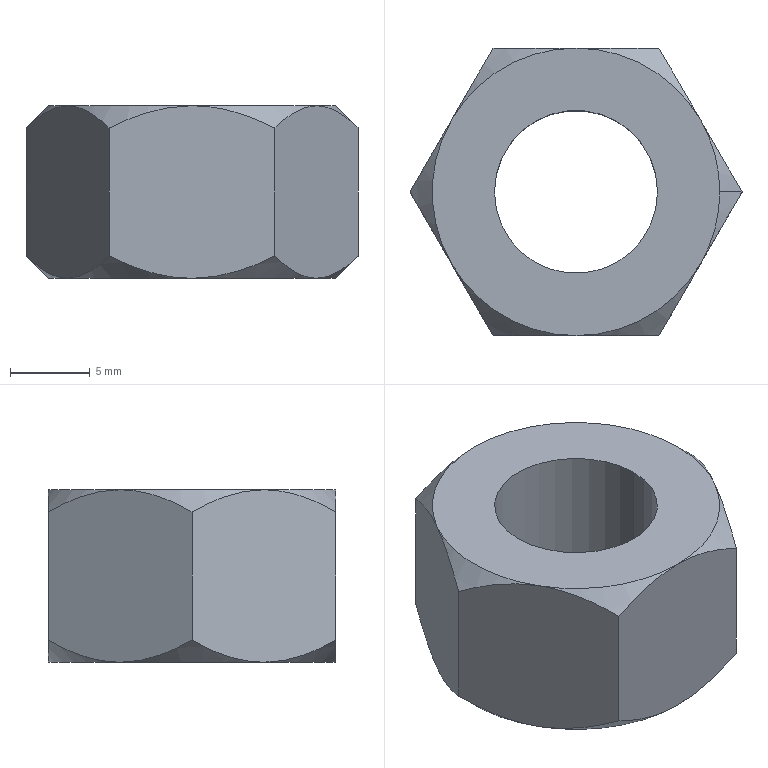Part | SolidWorks | features Extrusion 1, MirrorPattern 1, RevCutThin 1 | 1 solid | 24 faces | box 20.785 x 18 x 10.8 mm | volume 2126 mm3 | cone 14 | plane 8 | cylinder 2 | commonest cylinder face diameters 10.2 x2
STEP:
#1=CARTESIAN_POINT('',(9.,0.,10.8));
#2=VERTEX_POINT('',#1);
#3=CARTESIAN_POINT('',(7.794,4.5,10.8));
#4=VERTEX_POINT('',#3);
#5=CARTESIAN_POINT('',(0.,0.,10.8));
#6=DIRECTION('',(0.,0.,1.));
#7=DIRECTION('',(1.,0.,0.));
#8=AXIS2_PLACEMENT_3D('',#5,#6,#7);
#9=CIRCLE('',#8,9.);
#10=EDGE_CURVE('',#2,#4,#9,.T.);
#11=ORIENTED_EDGE('',*,*,#10,.F.);
#12=CARTESIAN_POINT('',(10.392,0.,9.408));
#13=VERTEX_POINT('',#12);
#14=CARTESIAN_POINT('',(9.,0.,10.8));
#15=DIRECTION('',(0.7071,0.,-0.7071));
#16=VECTOR('',#15,1000.);
#17=LINE('',#14,#16);
#18=EDGE_CURVE('',#2,#13,#17,.T.);
#19=ORIENTED_EDGE('',*,*,#18,.T.);
#20=CARTESIAN_POINT('',(7.794,4.5,10.8));
#21=CARTESIAN_POINT('',(8.246,3.717,10.8));
#22=CARTESIAN_POINT('',(8.69,2.948,10.662));
#23=CARTESIAN_POINT('',(9.566,1.43,10.164));
#24=CARTESIAN_POINT('',(9.985,0.7048,9.815));
#25=CARTESIAN_POINT('',(10.392,0.,9.408));
#26=B_SPLINE_CURVE_WITH_KNOTS('',3,(#20,#21,#22,#23,#24,#25),.UNSPECIFIED.,.F.,.F.,(4,2,4),(0.005387,0.008061,0.01074),.UNSPECIFIED.);
#27=EDGE_CURVE('',#4,#13,#26,.T.);
#28=ORIENTED_EDGE('',*,*,#27,.F.);
#29=EDGE_LOOP('',(#11,#19,#28));
#30=FACE_OUTER_BOUND('',#29,.T.);
#31=CARTESIAN_POINT('',(0.,0.,10.8));
#32=DIRECTION('',(0.,0.,-1.));
#33=DIRECTION('',(1.,0.,0.));
#34=AXIS2_PLACEMENT_3D('',#31,#32,#33);
#35=CONICAL_SURFACE('',#34,9.,0.7854);
#36=ADVANCED_FACE('',(#30),#35,.T.);
#37=CARTESIAN_POINT('',(7.794,-4.5,0.));
#38=VERTEX_POINT('',#37);
#39=CARTESIAN_POINT('',(9.,0.,0.));
#40=VERTEX_POINT('',#39);
#41=CARTESIAN_POINT('',(0.,0.,0.));
#42=DIRECTION('',(0.,0.,1.));
#43=DIRECTION('',(1.,0.,0.));
#44=AXIS2_PLACEMENT_3D('',#41,#42,#43);
#45=CIRCLE('',#44,9.);
#46=EDGE_CURVE('',#38,#40,#45,.T.);
#47=ORIENTED_EDGE('',*,*,#46,.T.);
#48=CARTESIAN_POINT('',(10.392,0.,1.392));
#49=VERTEX_POINT('',#48);
#50=CARTESIAN_POINT('',(9.,0.,0.));
#51=DIRECTION('',(0.7071,0.,0.7071));
#52=VECTOR('',#51,1000.);
#53=LINE('',#50,#52);
#54=EDGE_CURVE('',#40,#49,#53,.T.);
#55=ORIENTED_EDGE('',*,*,#54,.T.);
#56=CARTESIAN_POINT('',(7.794,-4.5,0.));
#57=CARTESIAN_POINT('',(8.246,-3.717,0.));
#58=CARTESIAN_POINT('',(8.69,-2.948,0.1382));
#59=CARTESIAN_POINT('',(9.566,-1.43,0.6363));
#60=CARTESIAN_POINT('',(9.985,-0.7048,0.9854));
#61=CARTESIAN_POINT('',(10.392,0.,1.392));
#62=B_SPLINE_CURVE_WITH_KNOTS('',3,(#56,#57,#58,#59,#60,#61),.UNSPECIFIED.,.F.,.F.,(4,2,4),(0.005387,0.008061,0.01074),.UNSPECIFIED.);
#63=EDGE_CURVE('',#38,#49,#62,.T.);
#64=ORIENTED_EDGE('',*,*,#63,.F.);
#65=EDGE_LOOP('',(#47,#55,#64));
#66=FACE_OUTER_BOUND('',#65,.T.);
#67=CARTESIAN_POINT('',(0.,0.,0.));
#68=DIRECTION('',(0.,0.,1.));
#69=DIRECTION('',(1.,0.,0.));
#70=AXIS2_PLACEMENT_3D('',#67,#68,#69);
#71=CONICAL_SURFACE('',#70,9.,0.7854);
#72=ADVANCED_FACE('',(#66),#71,.T.);
#73=CARTESIAN_POINT('',(-5.1,0.,10.8));
#74=VERTEX_POINT('',#73);
#75=CARTESIAN_POINT('',(5.1,0.,10.8));
#76=VERTEX_POINT('',#75);
#77=CARTESIAN_POINT('',(0.,0.,10.8));
#78=DIRECTION('',(0.,0.,1.));
#79=DIRECTION('',(1.,0.,0.));
#80=AXIS2_PLACEMENT_3D('',#77,#78,#79);
#81=CIRCLE('',#80,5.1);
#82=EDGE_CURVE('',#74,#76,#81,.T.);
#83=ORIENTED_EDGE('',*,*,#82,.T.);
#84=CARTESIAN_POINT('',(5.1,0.,0.));
#85=VERTEX_POINT('',#84);
#86=CARTESIAN_POINT('',(5.1,0.,10.8));
#87=DIRECTION('',(0.,0.,-1.));
#88=VECTOR('',#87,1000.);
#89=LINE('',#86,#88);
#90=EDGE_CURVE('',#76,#85,#89,.T.);
#91=ORIENTED_EDGE('',*,*,#90,.T.);
#92=CARTESIAN_POINT('',(-5.1,0.,0.));
#93=VERTEX_POINT('',#92);
#94=CARTESIAN_POINT('',(0.,0.,0.));
#95=DIRECTION('',(0.,0.,1.));
#96=DIRECTION('',(1.,0.,0.));
#97=AXIS2_PLACEMENT_3D('',#94,#95,#96);
#98=CIRCLE('',#97,5.1);
#99=EDGE_CURVE('',#93,#85,#98,.T.);
#100=ORIENTED_EDGE('',*,*,#99,.F.);
#101=CARTESIAN_POINT('',(-5.1,0.,10.8));
#102=DIRECTION('',(0.,0.,-1.));
#103=VECTOR('',#102,1000.);
#104=LINE('',#101,#103);
#105=EDGE_CURVE('',#74,#93,#104,.T.);
#106=ORIENTED_EDGE('',*,*,#105,.F.);
#107=EDGE_LOOP('',(#83,#91,#100,#106));
#108=FACE_OUTER_BOUND('',#107,.T.);
#109=CARTESIAN_POINT('',(0.,0.,10.8));
#110=DIRECTION('',(0.,0.,-1.));
#111=DIRECTION('',(-1.,0.,0.));
#112=AXIS2_PLACEMENT_3D('',#109,#110,#111);
#113=CYLINDRICAL_SURFACE('',#112,5.1);
#114=ADVANCED_FACE('',(#108),#113,.F.);
#115=CARTESIAN_POINT('',(0.,-9.,10.8));
#116=VERTEX_POINT('',#115);
#117=CARTESIAN_POINT('',(7.794,-4.5,10.8));
#118=VERTEX_POINT('',#117);
#119=CARTESIAN_POINT('',(0.,0.,10.8));
#120=DIRECTION('',(0.,0.,1.));
#121=DIRECTION('',(1.,0.,0.));
#122=AXIS2_PLACEMENT_3D('',#119,#120,#121);
#123=CIRCLE('',#122,9.);
#124=EDGE_CURVE('',#116,#118,#123,.T.);
#125=ORIENTED_EDGE('',*,*,#124,.T.);
#126=CARTESIAN_POINT('',(0.,0.,10.8));
#127=DIRECTION('',(0.,0.,1.));
#128=DIRECTION('',(1.,0.,0.));
#129=AXIS2_PLACEMENT_3D('',#126,#127,#128);
#130=CIRCLE('',#129,9.);
#131=EDGE_CURVE('',#118,#2,#130,.T.);
#132=ORIENTED_EDGE('',*,*,#131,.T.);
#133=ORIENTED_EDGE('',*,*,#10,.T.);
#134=CARTESIAN_POINT('',(0.,9.,10.8));
#135=VERTEX_POINT('',#134);
#136=CARTESIAN_POINT('',(0.,0.,10.8));
#137=DIRECTION('',(0.,0.,1.));
#138=DIRECTION('',(1.,0.,0.));
#139=AXIS2_PLACEMENT_3D('',#136,#137,#138);
#140=CIRCLE('',#139,9.);
#141=EDGE_CURVE('',#4,#135,#140,.T.);
#142=ORIENTED_EDGE('',*,*,#141,.T.);
#143=CARTESIAN_POINT('',(-7.794,4.5,10.8));
#144=VERTEX_POINT('',#143);
#145=CARTESIAN_POINT('',(0.,0.,10.8));
#146=DIRECTION('',(0.,0.,1.));
#147=DIRECTION('',(1.,0.,0.));
#148=AXIS2_PLACEMENT_3D('',#145,#146,#147);
#149=CIRCLE('',#148,9.);
#150=EDGE_CURVE('',#135,#144,#149,.T.);
#151=ORIENTED_EDGE('',*,*,#150,.T.);
#152=CARTESIAN_POINT('',(-7.794,-4.5,10.8));
#153=VERTEX_POINT('',#152);
#154=CARTESIAN_POINT('',(0.,0.,10.8));
#155=DIRECTION('',(0.,0.,1.));
#156=DIRECTION('',(1.,0.,0.));
#157=AXIS2_PLACEMENT_3D('',#154,#155,#156);
#158=CIRCLE('',#157,9.);
#159=EDGE_CURVE('',#144,#153,#158,.T.);
#160=ORIENTED_EDGE('',*,*,#159,.T.);
#161=CARTESIAN_POINT('',(0.,0.,10.8));
#162=DIRECTION('',(0.,0.,1.));
#163=DIRECTION('',(1.,0.,0.));
#164=AXIS2_PLACEMENT_3D('',#161,#162,#163);
#165=CIRCLE('',#164,9.);
#166=EDGE_CURVE('',#153,#116,#165,.T.);
#167=ORIENTED_EDGE('',*,*,#166,.T.);
#168=EDGE_LOOP('',(#125,#132,#133,#142,#151,#160,#167));
#169=FACE_OUTER_BOUND('',#168,.T.);
#170=ORIENTED_EDGE('',*,*,#82,.F.);
#171=CARTESIAN_POINT('',(0.,0.,10.8));
#172=DIRECTION('',(0.,0.,1.));
#173=DIRECTION('',(1.,0.,0.));
#174=AXIS2_PLACEMENT_3D('',#171,#172,#173);
#175=CIRCLE('',#174,5.1);
#176=EDGE_CURVE('',#76,#74,#175,.T.);
#177=ORIENTED_EDGE('',*,*,#176,.F.);
#178=EDGE_LOOP('',(#170,#177));
#179=FACE_BOUND('',#178,.T.);
#180=CARTESIAN_POINT('',(0.,0.,10.8));
#181=DIRECTION('',(0.,0.,1.));
#182=DIRECTION('',(1.,0.,0.));
#183=AXIS2_PLACEMENT_3D('',#180,#181,#182);
#184=PLANE('',#183);
#185=ADVANCED_FACE('',(#169,#179),#184,.T.);
#186=ORIENTED_EDGE('',*,*,#46,.F.);
#187=CARTESIAN_POINT('',(0.,-9.,0.));
#188=VERTEX_POINT('',#187);
#189=CARTESIAN_POINT('',(0.,0.,0.));
#190=DIRECTION('',(0.,0.,1.));
#191=DIRECTION('',(1.,0.,0.));
#192=AXIS2_PLACEMENT_3D('',#189,#190,#191);
#193=CIRCLE('',#192,9.);
#194=EDGE_CURVE('',#188,#38,#193,.T.);
#195=ORIENTED_EDGE('',*,*,#194,.F.);
#196=CARTESIAN_POINT('',(-7.794,-4.5,0.));
#197=VERTEX_POINT('',#196);
#198=CARTESIAN_POINT('',(0.,0.,0.));
#199=DIRECTION('',(0.,0.,1.));
#200=DIRECTION('',(1.,0.,0.));
#201=AXIS2_PLACEMENT_3D('',#198,#199,#200);
#202=CIRCLE('',#201,9.);
#203=EDGE_CURVE('',#197,#188,#202,.T.);
#204=ORIENTED_EDGE('',*,*,#203,.F.);
#205=CARTESIAN_POINT('',(-7.794,4.5,0.));
#206=VERTEX_POINT('',#205);
#207=CARTESIAN_POINT('',(0.,0.,0.));
#208=DIRECTION('',(0.,0.,1.));
#209=DIRECTION('',(1.,0.,0.));
#210=AXIS2_PLACEMENT_3D('',#207,#208,#209);
#211=CIRCLE('',#210,9.);
#212=EDGE_CURVE('',#206,#197,#211,.T.);
#213=ORIENTED_EDGE('',*,*,#212,.F.);
#214=CARTESIAN_POINT('',(0.,9.,0.));
#215=VERTEX_POINT('',#214);
#216=CARTESIAN_POINT('',(0.,0.,0.));
#217=DIRECTION('',(0.,0.,1.));
#218=DIRECTION('',(1.,0.,0.));
#219=AXIS2_PLACEMENT_3D('',#216,#217,#218);
#220=CIRCLE('',#219,9.);
#221=EDGE_CURVE('',#215,#206,#220,.T.);
#222=ORIENTED_EDGE('',*,*,#221,.F.);
#223=CARTESIAN_POINT('',(7.794,4.5,0.));
#224=VERTEX_POINT('',#223);
#225=CARTESIAN_POINT('',(0.,0.,0.));
#226=DIRECTION('',(0.,0.,1.));
#227=DIRECTION('',(1.,0.,0.));
#228=AXIS2_PLACEMENT_3D('',#225,#226,#227);
#229=CIRCLE('',#228,9.);
#230=EDGE_CURVE('',#224,#215,#229,.T.);
#231=ORIENTED_EDGE('',*,*,#230,.F.);
#232=CARTESIAN_POINT('',(0.,0.,0.));
#233=DIRECTION('',(0.,0.,1.));
#234=DIRECTION('',(1.,0.,0.));
#235=AXIS2_PLACEMENT_3D('',#232,#233,#234);
#236=CIRCLE('',#235,9.);
#237=EDGE_CURVE('',#40,#224,#236,.T.);
#238=ORIENTED_EDGE('',*,*,#237,.F.);
#239=EDGE_LOOP('',(#186,#195,#204,#213,#222,#231,#238));
#240=FACE_OUTER_BOUND('',#239,.T.);
#241=ORIENTED_EDGE('',*,*,#99,.T.);
#242=CARTESIAN_POINT('',(0.,0.,0.));
#243=DIRECTION('',(0.,0.,1.));
#244=DIRECTION('',(1.,0.,0.));
#245=AXIS2_PLACEMENT_3D('',#242,#243,#244);
#246=CIRCLE('',#245,5.1);
#247=EDGE_CURVE('',#85,#93,#246,.T.);
#248=ORIENTED_EDGE('',*,*,#247,.T.);
#249=EDGE_LOOP('',(#241,#248));
#250=FACE_BOUND('',#249,.T.);
#251=CARTESIAN_POINT('',(0.,0.,0.));
#252=DIRECTION('',(0.,0.,1.));
#253=DIRECTION('',(1.,0.,0.));
#254=AXIS2_PLACEMENT_3D('',#251,#252,#253);
#255=PLANE('',#254);
#256=ADVANCED_FACE('',(#240,#250),#255,.F.);
#257=CARTESIAN_POINT('',(-5.196,9.,9.408));
#258=VERTEX_POINT('',#257);
#259=CARTESIAN_POINT('',(-5.196,9.,1.392));
#260=VERTEX_POINT('',#259);
#261=CARTESIAN_POINT('',(-5.196,9.,10.8));
#262=DIRECTION('',(0.,0.,-1.));
#263=VECTOR('',#262,1000.);
#264=LINE('',#261,#263);
#265=EDGE_CURVE('',#258,#260,#264,.T.);
#266=ORIENTED_EDGE('',*,*,#265,.F.);
#267=CARTESIAN_POINT('',(-5.196,9.,9.408));
#268=CARTESIAN_POINT('',(-4.793,9.,9.609));
#269=CARTESIAN_POINT('',(-4.38,9.,9.798));
#270=CARTESIAN_POINT('',(-3.536,9.,10.138));
#271=CARTESIAN_POINT('',(-3.109,9.,10.287));
#272=CARTESIAN_POINT('',(-2.244,9.,10.534));
#273=CARTESIAN_POINT('',(-1.586,9.,10.68));
#274=CARTESIAN_POINT('',(-0.9111,9.,10.757));
#275=CARTESIAN_POINT('',(-0.4575,9.,10.791));
#276=CARTESIAN_POINT('',(-0.2277,9.,10.8));
#277=CARTESIAN_POINT('',(0.,9.,10.8));
#278=B_SPLINE_CURVE_WITH_KNOTS('',3,(#267,#268,#269,#270,#271,#272,#273,#274,#275,#276,#277),.UNSPECIFIED.,.F.,.F.,(4,2,2,1,2,4),(0.009591,0.01093,0.01227,0.01361,0.01429,0.01496),.UNSPECIFIED.);
#279=EDGE_CURVE('',#258,#135,#278,.T.);
#280=ORIENTED_EDGE('',*,*,#279,.T.);
#281=CARTESIAN_POINT('',(5.196,9.,9.408));
#282=VERTEX_POINT('',#281);
#283=CARTESIAN_POINT('',(0.,9.,10.8));
#284=CARTESIAN_POINT('',(0.9123,9.,10.8));
#285=CARTESIAN_POINT('',(1.802,9.,10.66));
#286=CARTESIAN_POINT('',(3.109,9.,10.287));
#287=CARTESIAN_POINT('',(3.543,9.,10.136));
#288=CARTESIAN_POINT('',(4.384,9.,9.797));
#289=CARTESIAN_POINT('',(4.794,9.,9.609));
#290=CARTESIAN_POINT('',(5.196,9.,9.408));
#291=B_SPLINE_CURVE_WITH_KNOTS('',3,(#283,#284,#285,#286,#287,#288,#289,#290),.UNSPECIFIED.,.F.,.F.,(4,2,2,4),(0.01496,0.01764,0.01899,0.02033),.UNSPECIFIED.);
#292=EDGE_CURVE('',#135,#282,#291,.T.);
#293=ORIENTED_EDGE('',*,*,#292,.T.);
#294=CARTESIAN_POINT('',(5.196,9.,1.392));
#295=VERTEX_POINT('',#294);
#296=CARTESIAN_POINT('',(5.196,9.,10.8));
#297=DIRECTION('',(0.,0.,-1.));
#298=VECTOR('',#297,1000.);
#299=LINE('',#296,#298);
#300=EDGE_CURVE('',#282,#295,#299,.T.);
#301=ORIENTED_EDGE('',*,*,#300,.T.);
#302=CARTESIAN_POINT('',(5.196,9.,1.392));
#303=CARTESIAN_POINT('',(4.794,9.,1.191));
#304=CARTESIAN_POINT('',(4.384,9.,1.003));
#305=CARTESIAN_POINT('',(3.543,9.,0.6644));
#306=CARTESIAN_POINT('',(3.109,9.,0.5127));
#307=CARTESIAN_POINT('',(1.802,9.,0.1404));
#308=CARTESIAN_POINT('',(0.9123,9.,0.));
#309=CARTESIAN_POINT('',(0.,9.,0.));
#310=B_SPLINE_CURVE_WITH_KNOTS('',3,(#302,#303,#304,#305,#306,#307,#308,#309),.UNSPECIFIED.,.F.,.F.,(4,2,2,4),(0.005444,0.006791,0.008139,0.01083),.UNSPECIFIED.);
#311=EDGE_CURVE('',#295,#215,#310,.T.);
#312=ORIENTED_EDGE('',*,*,#311,.T.);
#313=CARTESIAN_POINT('',(0.,9.,0.));
#314=CARTESIAN_POINT('',(-0.2277,9.,0.));
#315=CARTESIAN_POINT('',(-0.4575,9.,0.008784));
#316=CARTESIAN_POINT('',(-0.9111,9.,0.04317));
#317=CARTESIAN_POINT('',(-1.586,9.,0.1198));
#318=CARTESIAN_POINT('',(-2.244,9.,0.2662));
#319=CARTESIAN_POINT('',(-3.109,9.,0.513));
#320=CARTESIAN_POINT('',(-3.536,9.,0.6621));
#321=CARTESIAN_POINT('',(-4.38,9.,1.002));
#322=CARTESIAN_POINT('',(-4.793,9.,1.191));
#323=CARTESIAN_POINT('',(-5.196,9.,1.392));
#324=B_SPLINE_CURVE_WITH_KNOTS('',3,(#313,#314,#315,#316,#317,#318,#319,#320,#321,#322,#323),.UNSPECIFIED.,.F.,.F.,(4,2,1,2,2,4),(0.01083,0.01151,0.01218,0.01352,0.01487,0.01622),.UNSPECIFIED.);
#325=EDGE_CURVE('',#215,#260,#324,.T.);
#326=ORIENTED_EDGE('',*,*,#325,.T.);
#327=EDGE_LOOP('',(#266,#280,#293,#301,#312,#326));
#328=FACE_OUTER_BOUND('',#327,.T.);
#329=CARTESIAN_POINT('',(5.196,9.,10.8));
#330=DIRECTION('',(0.,-1.,0.));
#331=DIRECTION('',(0.,0.,-1.));
#332=AXIS2_PLACEMENT_3D('',#329,#330,#331);
#333=PLANE('',#332);
#334=ADVANCED_FACE('',(#328),#333,.F.);
#335=CARTESIAN_POINT('',(-10.392,0.,9.408));
#336=VERTEX_POINT('',#335);
#337=CARTESIAN_POINT('',(-10.392,0.,1.392));
#338=VERTEX_POINT('',#337);
#339=CARTESIAN_POINT('',(-10.392,0.,10.8));
#340=DIRECTION('',(0.,0.,-1.));
#341=VECTOR('',#340,1000.);
#342=LINE('',#339,#341);
#343=EDGE_CURVE('',#336,#338,#342,.T.);
#344=ORIENTED_EDGE('',*,*,#343,.F.);
#345=CARTESIAN_POINT('',(-10.392,0.,9.408));
#346=CARTESIAN_POINT('',(-9.985,0.7057,9.815));
#347=CARTESIAN_POINT('',(-9.568,1.427,10.161));
#348=CARTESIAN_POINT('',(-8.921,2.549,10.531));
#349=CARTESIAN_POINT('',(-8.701,2.929,10.63));
#350=CARTESIAN_POINT('',(-8.253,3.706,10.764));
#351=CARTESIAN_POINT('',(-8.022,4.106,10.8));
#352=CARTESIAN_POINT('',(-7.794,4.5,10.8));
#353=B_SPLINE_CURVE_WITH_KNOTS('',3,(#345,#346,#347,#348,#349,#350,#351,#352),.UNSPECIFIED.,.F.,.F.,(4,2,2,4),(0.000000254,0.002693,0.00404,0.005387),.UNSPECIFIED.);
#354=EDGE_CURVE('',#336,#144,#353,.T.);
#355=ORIENTED_EDGE('',*,*,#354,.T.);
#356=CARTESIAN_POINT('',(-7.794,4.5,10.8));
#357=CARTESIAN_POINT('',(-7.342,5.283,10.8));
#358=CARTESIAN_POINT('',(-6.898,6.052,10.662));
#359=CARTESIAN_POINT('',(-6.022,7.57,10.164));
#360=CARTESIAN_POINT('',(-5.603,8.295,9.815));
#361=CARTESIAN_POINT('',(-5.196,9.,9.408));
#362=B_SPLINE_CURVE_WITH_KNOTS('',3,(#356,#357,#358,#359,#360,#361),.UNSPECIFIED.,.F.,.F.,(4,2,4),(0.005387,0.008061,0.01074),.UNSPECIFIED.);
#363=EDGE_CURVE('',#144,#258,#362,.T.);
#364=ORIENTED_EDGE('',*,*,#363,.T.);
#365=ORIENTED_EDGE('',*,*,#265,.T.);
#366=CARTESIAN_POINT('',(-5.196,9.,1.392));
#367=CARTESIAN_POINT('',(-5.604,8.294,0.9849));
#368=CARTESIAN_POINT('',(-6.02,7.573,0.6387));
#369=CARTESIAN_POINT('',(-6.668,6.451,0.2685));
#370=CARTESIAN_POINT('',(-6.887,6.071,0.1703));
#371=CARTESIAN_POINT('',(-7.336,5.294,0.03572));
#372=CARTESIAN_POINT('',(-7.567,4.894,0.));
#373=CARTESIAN_POINT('',(-7.794,4.5,0.));
#374=B_SPLINE_CURVE_WITH_KNOTS('',3,(#366,#367,#368,#369,#370,#371,#372,#373),.UNSPECIFIED.,.F.,.F.,(4,2,2,4),(0.000000254,0.002693,0.00404,0.005387),.UNSPECIFIED.);
#375=EDGE_CURVE('',#260,#206,#374,.T.);
#376=ORIENTED_EDGE('',*,*,#375,.T.);
#377=CARTESIAN_POINT('',(-7.794,4.5,0.));
#378=CARTESIAN_POINT('',(-8.246,3.717,0.));
#379=CARTESIAN_POINT('',(-8.69,2.948,0.1382));
#380=CARTESIAN_POINT('',(-9.566,1.43,0.6363));
#381=CARTESIAN_POINT('',(-9.985,0.7048,0.9854));
#382=CARTESIAN_POINT('',(-10.392,0.,1.392));
#383=B_SPLINE_CURVE_WITH_KNOTS('',3,(#377,#378,#379,#380,#381,#382),.UNSPECIFIED.,.F.,.F.,(4,2,4),(0.005387,0.008061,0.01074),.UNSPECIFIED.);
#384=EDGE_CURVE('',#206,#338,#383,.T.);
#385=ORIENTED_EDGE('',*,*,#384,.T.);
#386=EDGE_LOOP('',(#344,#355,#364,#365,#376,#385));
#387=FACE_OUTER_BOUND('',#386,.T.);
#388=CARTESIAN_POINT('',(-5.196,9.,10.8));
#389=DIRECTION('',(0.866,-0.5,0.));
#390=DIRECTION('',(0.5,0.866,0.));
#391=AXIS2_PLACEMENT_3D('',#388,#389,#390);
#392=PLANE('',#391);
#393=ADVANCED_FACE('',(#387),#392,.F.);
#394=CARTESIAN_POINT('',(-5.196,-9.,9.408));
#395=VERTEX_POINT('',#394);
#396=CARTESIAN_POINT('',(-5.196,-9.,1.392));
#397=VERTEX_POINT('',#396);
#398=CARTESIAN_POINT('',(-5.196,-9.,10.8));
#399=DIRECTION('',(0.,0.,-1.));
#400=VECTOR('',#399,1000.);
#401=LINE('',#398,#400);
#402=EDGE_CURVE('',#395,#397,#401,.T.);
#403=ORIENTED_EDGE('',*,*,#402,.F.);
#404=CARTESIAN_POINT('',(-5.196,-9.,9.408));
#405=CARTESIAN_POINT('',(-5.604,-8.294,9.815));
#406=CARTESIAN_POINT('',(-6.02,-7.573,10.161));
#407=CARTESIAN_POINT('',(-6.668,-6.451,10.531));
#408=CARTESIAN_POINT('',(-6.887,-6.071,10.63));
#409=CARTESIAN_POINT('',(-7.336,-5.294,10.764));
#410=CARTESIAN_POINT('',(-7.567,-4.894,10.8));
#411=CARTESIAN_POINT('',(-7.794,-4.5,10.8));
#412=B_SPLINE_CURVE_WITH_KNOTS('',3,(#404,#405,#406,#407,#408,#409,#410,#411),.UNSPECIFIED.,.F.,.F.,(4,2,2,4),(0.000000254,0.002693,0.00404,0.005387),.UNSPECIFIED.);
#413=EDGE_CURVE('',#395,#153,#412,.T.);
#414=ORIENTED_EDGE('',*,*,#413,.T.);
#415=CARTESIAN_POINT('',(-7.794,-4.5,10.8));
#416=CARTESIAN_POINT('',(-8.246,-3.717,10.8));
#417=CARTESIAN_POINT('',(-8.69,-2.948,10.662));
#418=CARTESIAN_POINT('',(-9.566,-1.43,10.164));
#419=CARTESIAN_POINT('',(-9.985,-0.7048,9.815));
#420=CARTESIAN_POINT('',(-10.392,0.,9.408));
#421=B_SPLINE_CURVE_WITH_KNOTS('',3,(#415,#416,#417,#418,#419,#420),.UNSPECIFIED.,.F.,.F.,(4,2,4),(0.005387,0.008061,0.01074),.UNSPECIFIED.);
#422=EDGE_CURVE('',#153,#336,#421,.T.);
#423=ORIENTED_EDGE('',*,*,#422,.T.);
#424=ORIENTED_EDGE('',*,*,#343,.T.);
#425=CARTESIAN_POINT('',(-10.392,0.,1.392));
#426=CARTESIAN_POINT('',(-9.985,-0.7057,0.9849));
#427=CARTESIAN_POINT('',(-9.568,-1.427,0.6387));
#428=CARTESIAN_POINT('',(-8.921,-2.549,0.2685));
#429=CARTESIAN_POINT('',(-8.701,-2.929,0.1703));
#430=CARTESIAN_POINT('',(-8.253,-3.706,0.03572));
#431=CARTESIAN_POINT('',(-8.022,-4.106,0.));
#432=CARTESIAN_POINT('',(-7.794,-4.5,0.));
#433=B_SPLINE_CURVE_WITH_KNOTS('',3,(#425,#426,#427,#428,#429,#430,#431,#432),.UNSPECIFIED.,.F.,.F.,(4,2,2,4),(0.000000254,0.002693,0.00404,0.005387),.UNSPECIFIED.);
#434=EDGE_CURVE('',#338,#197,#433,.T.);
#435=ORIENTED_EDGE('',*,*,#434,.T.);
#436=CARTESIAN_POINT('',(-7.794,-4.5,0.));
#437=CARTESIAN_POINT('',(-7.342,-5.283,0.));
#438=CARTESIAN_POINT('',(-6.898,-6.052,0.1382));
#439=CARTESIAN_POINT('',(-6.022,-7.57,0.6363));
#440=CARTESIAN_POINT('',(-5.603,-8.295,0.9854));
#441=CARTESIAN_POINT('',(-5.196,-9.,1.392));
#442=B_SPLINE_CURVE_WITH_KNOTS('',3,(#436,#437,#438,#439,#440,#441),.UNSPECIFIED.,.F.,.F.,(4,2,4),(0.005387,0.008061,0.01074),.UNSPECIFIED.);
#443=EDGE_CURVE('',#197,#397,#442,.T.);
#444=ORIENTED_EDGE('',*,*,#443,.T.);
#445=EDGE_LOOP('',(#403,#414,#423,#424,#435,#444));
#446=FACE_OUTER_BOUND('',#445,.T.);
#447=CARTESIAN_POINT('',(-10.392,0.,10.8));
#448=DIRECTION('',(0.866,0.5,0.));
#449=DIRECTION('',(-0.5,0.866,0.));
#450=AXIS2_PLACEMENT_3D('',#447,#448,#449);
#451=PLANE('',#450);
#452=ADVANCED_FACE('',(#446),#451,.F.);
#453=CARTESIAN_POINT('',(5.196,-9.,9.408));
#454=VERTEX_POINT('',#453);
#455=CARTESIAN_POINT('',(5.196,-9.,1.392));
#456=VERTEX_POINT('',#455);
#457=CARTESIAN_POINT('',(5.196,-9.,10.8));
#458=DIRECTION('',(0.,0.,-1.));
#459=VECTOR('',#458,1000.);
#460=LINE('',#457,#459);
#461=EDGE_CURVE('',#454,#456,#460,.T.);
#462=ORIENTED_EDGE('',*,*,#461,.F.);
#463=CARTESIAN_POINT('',(5.196,-9.,9.408));
#464=CARTESIAN_POINT('',(4.794,-9.,9.609));
#465=CARTESIAN_POINT('',(4.384,-9.,9.797));
#466=CARTESIAN_POINT('',(3.543,-9.,10.136));
#467=CARTESIAN_POINT('',(3.109,-9.,10.287));
#468=CARTESIAN_POINT('',(1.802,-9.,10.66));
#469=CARTESIAN_POINT('',(0.9123,-9.,10.8));
#470=CARTESIAN_POINT('',(0.,-9.,10.8));
#471=B_SPLINE_CURVE_WITH_KNOTS('',3,(#463,#464,#465,#466,#467,#468,#469,#470),.UNSPECIFIED.,.F.,.F.,(4,2,2,4),(0.005444,0.006791,0.008139,0.01083),.UNSPECIFIED.);
#472=EDGE_CURVE('',#454,#116,#471,.T.);
#473=ORIENTED_EDGE('',*,*,#472,.T.);
#474=CARTESIAN_POINT('',(0.,-9.,10.8));
#475=CARTESIAN_POINT('',(-0.2277,-9.,10.8));
#476=CARTESIAN_POINT('',(-0.4575,-9.,10.791));
#477=CARTESIAN_POINT('',(-0.9111,-9.,10.757));
#478=CARTESIAN_POINT('',(-1.586,-9.,10.68));
#479=CARTESIAN_POINT('',(-2.244,-9.,10.534));
#480=CARTESIAN_POINT('',(-3.109,-9.,10.287));
#481=CARTESIAN_POINT('',(-3.536,-9.,10.138));
#482=CARTESIAN_POINT('',(-4.38,-9.,9.798));
#483=CARTESIAN_POINT('',(-4.793,-9.,9.609));
#484=CARTESIAN_POINT('',(-5.196,-9.,9.408));
#485=B_SPLINE_CURVE_WITH_KNOTS('',3,(#474,#475,#476,#477,#478,#479,#480,#481,#482,#483,#484),.UNSPECIFIED.,.F.,.F.,(4,2,1,2,2,4),(0.01083,0.01151,0.01218,0.01352,0.01487,0.01622),.UNSPECIFIED.);
#486=EDGE_CURVE('',#116,#395,#485,.T.);
#487=ORIENTED_EDGE('',*,*,#486,.T.);
#488=ORIENTED_EDGE('',*,*,#402,.T.);
#489=CARTESIAN_POINT('',(-5.196,-9.,1.392));
#490=CARTESIAN_POINT('',(-4.793,-9.,1.191));
#491=CARTESIAN_POINT('',(-4.38,-9.,1.002));
#492=CARTESIAN_POINT('',(-3.536,-9.,0.6621));
#493=CARTESIAN_POINT('',(-3.109,-9.,0.513));
#494=CARTESIAN_POINT('',(-2.244,-9.,0.2662));
#495=CARTESIAN_POINT('',(-1.586,-9.,0.1198));
#496=CARTESIAN_POINT('',(-0.9111,-9.,0.04317));
#497=CARTESIAN_POINT('',(-0.4575,-9.,0.008784));
#498=CARTESIAN_POINT('',(-0.2277,-9.,0.));
#499=CARTESIAN_POINT('',(0.,-9.,0.));
#500=B_SPLINE_CURVE_WITH_KNOTS('',3,(#489,#490,#491,#492,#493,#494,#495,#496,#497,#498,#499),.UNSPECIFIED.,.F.,.F.,(4,2,2,1,2,4),(0.009591,0.01093,0.01227,0.01361,0.01429,0.01496),.UNSPECIFIED.);
#501=EDGE_CURVE('',#397,#188,#500,.T.);
#502=ORIENTED_EDGE('',*,*,#501,.T.);
#503=CARTESIAN_POINT('',(0.,-9.,0.));
#504=CARTESIAN_POINT('',(0.9123,-9.,0.));
#505=CARTESIAN_POINT('',(1.802,-9.,0.1404));
#506=CARTESIAN_POINT('',(3.109,-9.,0.5127));
#507=CARTESIAN_POINT('',(3.543,-9.,0.6644));
#508=CARTESIAN_POINT('',(4.384,-9.,1.003));
#509=CARTESIAN_POINT('',(4.794,-9.,1.191));
#510=CARTESIAN_POINT('',(5.196,-9.,1.392));
#511=B_SPLINE_CURVE_WITH_KNOTS('',3,(#503,#504,#505,#506,#507,#508,#509,#510),.UNSPECIFIED.,.F.,.F.,(4,2,2,4),(0.01496,0.01764,0.01899,0.02033),.UNSPECIFIED.);
#512=EDGE_CURVE('',#188,#456,#511,.T.);
#513=ORIENTED_EDGE('',*,*,#512,.T.);
#514=EDGE_LOOP('',(#462,#473,#487,#488,#502,#513));
#515=FACE_OUTER_BOUND('',#514,.T.);
#516=CARTESIAN_POINT('',(-5.196,-9.,10.8));
#517=DIRECTION('',(0.,1.,0.));
#518=DIRECTION('',(0.,0.,1.));
#519=AXIS2_PLACEMENT_3D('',#516,#517,#518);
#520=PLANE('',#519);
#521=ADVANCED_FACE('',(#515),#520,.F.);
#522=CARTESIAN_POINT('',(10.392,0.,10.8));
#523=DIRECTION('',(0.,0.,-1.));
#524=VECTOR('',#523,1000.);
#525=LINE('',#522,#524);
#526=EDGE_CURVE('',#13,#49,#525,.T.);
#527=ORIENTED_EDGE('',*,*,#526,.F.);
#528=CARTESIAN_POINT('',(10.392,0.,9.408));
#529=CARTESIAN_POINT('',(9.985,-0.7057,9.815));
#530=CARTESIAN_POINT('',(9.568,-1.427,10.161));
#531=CARTESIAN_POINT('',(8.921,-2.549,10.531));
#532=CARTESIAN_POINT('',(8.701,-2.929,10.63));
#533=CARTESIAN_POINT('',(8.253,-3.706,10.764));
#534=CARTESIAN_POINT('',(8.022,-4.106,10.8));
#535=CARTESIAN_POINT('',(7.794,-4.5,10.8));
#536=B_SPLINE_CURVE_WITH_KNOTS('',3,(#528,#529,#530,#531,#532,#533,#534,#535),.UNSPECIFIED.,.F.,.F.,(4,2,2,4),(0.000000254,0.002693,0.00404,0.005387),.UNSPECIFIED.);
#537=EDGE_CURVE('',#13,#118,#536,.T.);
#538=ORIENTED_EDGE('',*,*,#537,.T.);
#539=CARTESIAN_POINT('',(7.794,-4.5,10.8));
#540=CARTESIAN_POINT('',(7.342,-5.283,10.8));
#541=CARTESIAN_POINT('',(6.898,-6.052,10.662));
#542=CARTESIAN_POINT('',(6.022,-7.57,10.164));
#543=CARTESIAN_POINT('',(5.603,-8.295,9.815));
#544=CARTESIAN_POINT('',(5.196,-9.,9.408));
#545=B_SPLINE_CURVE_WITH_KNOTS('',3,(#539,#540,#541,#542,#543,#544),.UNSPECIFIED.,.F.,.F.,(4,2,4),(0.005387,0.008061,0.01074),.UNSPECIFIED.);
#546=EDGE_CURVE('',#118,#454,#545,.T.);
#547=ORIENTED_EDGE('',*,*,#546,.T.);
#548=ORIENTED_EDGE('',*,*,#461,.T.);
#549=CARTESIAN_POINT('',(5.196,-9.,1.392));
#550=CARTESIAN_POINT('',(5.604,-8.294,0.9849));
#551=CARTESIAN_POINT('',(6.02,-7.573,0.6387));
#552=CARTESIAN_POINT('',(6.668,-6.451,0.2685));
#553=CARTESIAN_POINT('',(6.887,-6.071,0.1703));
#554=CARTESIAN_POINT('',(7.336,-5.294,0.03572));
#555=CARTESIAN_POINT('',(7.567,-4.894,0.));
#556=CARTESIAN_POINT('',(7.794,-4.5,0.));
#557=B_SPLINE_CURVE_WITH_KNOTS('',3,(#549,#550,#551,#552,#553,#554,#555,#556),.UNSPECIFIED.,.F.,.F.,(4,2,2,4),(0.000000254,0.002693,0.00404,0.005387),.UNSPECIFIED.);
#558=EDGE_CURVE('',#456,#38,#557,.T.);
#559=ORIENTED_EDGE('',*,*,#558,.T.);
#560=ORIENTED_EDGE('',*,*,#63,.T.);
#561=EDGE_LOOP('',(#527,#538,#547,#548,#559,#560));
#562=FACE_OUTER_BOUND('',#561,.T.);
#563=CARTESIAN_POINT('',(5.196,-9.,10.8));
#564=DIRECTION('',(-0.866,0.5,0.));
#565=DIRECTION('',(-0.5,-0.866,0.));
#566=AXIS2_PLACEMENT_3D('',#563,#564,#565);
#567=PLANE('',#566);
#568=ADVANCED_FACE('',(#562),#567,.F.);
#569=ORIENTED_EDGE('',*,*,#300,.F.);
#570=CARTESIAN_POINT('',(5.196,9.,9.408));
#571=CARTESIAN_POINT('',(5.604,8.294,9.815));
#572=CARTESIAN_POINT('',(6.02,7.573,10.161));
#573=CARTESIAN_POINT('',(6.668,6.451,10.531));
#574=CARTESIAN_POINT('',(6.887,6.071,10.63));
#575=CARTESIAN_POINT('',(7.336,5.294,10.764));
#576=CARTESIAN_POINT('',(7.567,4.894,10.8));
#577=CARTESIAN_POINT('',(7.794,4.5,10.8));
#578=B_SPLINE_CURVE_WITH_KNOTS('',3,(#570,#571,#572,#573,#574,#575,#576,#577),.UNSPECIFIED.,.F.,.F.,(4,2,2,4),(0.000000254,0.002693,0.00404,0.005387),.UNSPECIFIED.);
#579=EDGE_CURVE('',#282,#4,#578,.T.);
#580=ORIENTED_EDGE('',*,*,#579,.T.);
#581=ORIENTED_EDGE('',*,*,#27,.T.);
#582=ORIENTED_EDGE('',*,*,#526,.T.);
#583=CARTESIAN_POINT('',(10.392,0.,1.392));
#584=CARTESIAN_POINT('',(9.985,0.7057,0.9849));
#585=CARTESIAN_POINT('',(9.568,1.427,0.6387));
#586=CARTESIAN_POINT('',(8.921,2.549,0.2685));
#587=CARTESIAN_POINT('',(8.701,2.929,0.1703));
#588=CARTESIAN_POINT('',(8.253,3.706,0.03572));
#589=CARTESIAN_POINT('',(8.022,4.106,0.));
#590=CARTESIAN_POINT('',(7.794,4.5,0.));
#591=B_SPLINE_CURVE_WITH_KNOTS('',3,(#583,#584,#585,#586,#587,#588,#589,#590),.UNSPECIFIED.,.F.,.F.,(4,2,2,4),(0.000000254,0.002693,0.00404,0.005387),.UNSPECIFIED.);
#592=EDGE_CURVE('',#49,#224,#591,.T.);
#593=ORIENTED_EDGE('',*,*,#592,.T.);
#594=CARTESIAN_POINT('',(7.794,4.5,0.));
#595=CARTESIAN_POINT('',(7.342,5.283,0.));
#596=CARTESIAN_POINT('',(6.898,6.052,0.1382));
#597=CARTESIAN_POINT('',(6.022,7.57,0.6363));
#598=CARTESIAN_POINT('',(5.603,8.295,0.9854));
#599=CARTESIAN_POINT('',(5.196,9.,1.392));
#600=B_SPLINE_CURVE_WITH_KNOTS('',3,(#594,#595,#596,#597,#598,#599),.UNSPECIFIED.,.F.,.F.,(4,2,4),(0.005387,0.008061,0.01074),.UNSPECIFIED.);
#601=EDGE_CURVE('',#224,#295,#600,.T.);
#602=ORIENTED_EDGE('',*,*,#601,.T.);
#603=EDGE_LOOP('',(#569,#580,#581,#582,#593,#602));
#604=FACE_OUTER_BOUND('',#603,.T.);
#605=CARTESIAN_POINT('',(10.392,0.,10.8));
#606=DIRECTION('',(-0.866,-0.5,0.));
#607=DIRECTION('',(0.5,-0.866,0.));
#608=AXIS2_PLACEMENT_3D('',#605,#606,#607);
#609=PLANE('',#608);
#610=ADVANCED_FACE('',(#604),#609,.F.);
#611=ORIENTED_EDGE('',*,*,#90,.F.);
#612=ORIENTED_EDGE('',*,*,#176,.T.);
#613=ORIENTED_EDGE('',*,*,#105,.T.);
#614=ORIENTED_EDGE('',*,*,#247,.F.);
#615=EDGE_LOOP('',(#611,#612,#613,#614));
#616=FACE_OUTER_BOUND('',#615,.T.);
#617=CARTESIAN_POINT('',(0.,0.,10.8));
#618=DIRECTION('',(0.,0.,-1.));
#619=DIRECTION('',(-1.,0.,0.));
#620=AXIS2_PLACEMENT_3D('',#617,#618,#619);
#621=CYLINDRICAL_SURFACE('',#620,5.1);
#622=ADVANCED_FACE('',(#616),#621,.F.);
#623=ORIENTED_EDGE('',*,*,#601,.F.);
#624=ORIENTED_EDGE('',*,*,#230,.T.);
#625=ORIENTED_EDGE('',*,*,#311,.F.);
#626=EDGE_LOOP('',(#623,#624,#625));
#627=FACE_OUTER_BOUND('',#626,.T.);
#628=CARTESIAN_POINT('',(0.,0.,0.));
#629=DIRECTION('',(0.,0.,1.));
#630=DIRECTION('',(1.,0.,0.));
#631=AXIS2_PLACEMENT_3D('',#628,#629,#630);
#632=CONICAL_SURFACE('',#631,9.,0.7854);
#633=ADVANCED_FACE('',(#627),#632,.T.);
#634=ORIENTED_EDGE('',*,*,#54,.F.);
#635=ORIENTED_EDGE('',*,*,#237,.T.);
#636=ORIENTED_EDGE('',*,*,#592,.F.);
#637=EDGE_LOOP('',(#634,#635,#636));
#638=FACE_OUTER_BOUND('',#637,.T.);
#639=CARTESIAN_POINT('',(0.,0.,0.));
#640=DIRECTION('',(0.,0.,1.));
#641=DIRECTION('',(1.,0.,0.));
#642=AXIS2_PLACEMENT_3D('',#639,#640,#641);
#643=CONICAL_SURFACE('',#642,9.,0.7854);
#644=ADVANCED_FACE('',(#638),#643,.T.);
#645=ORIENTED_EDGE('',*,*,#194,.T.);
#646=ORIENTED_EDGE('',*,*,#558,.F.);
#647=ORIENTED_EDGE('',*,*,#512,.F.);
#648=EDGE_LOOP('',(#645,#646,#647));
#649=FACE_OUTER_BOUND('',#648,.T.);
#650=CARTESIAN_POINT('',(0.,0.,0.));
#651=DIRECTION('',(0.,0.,1.));
#652=DIRECTION('',(1.,0.,0.));
#653=AXIS2_PLACEMENT_3D('',#650,#651,#652);
#654=CONICAL_SURFACE('',#653,9.,0.7854);
#655=ADVANCED_FACE('',(#649),#654,.T.);
#656=ORIENTED_EDGE('',*,*,#203,.T.);
#657=ORIENTED_EDGE('',*,*,#501,.F.);
#658=ORIENTED_EDGE('',*,*,#443,.F.);
#659=EDGE_LOOP('',(#656,#657,#658));
#660=FACE_OUTER_BOUND('',#659,.T.);
#661=CARTESIAN_POINT('',(0.,0.,0.));
#662=DIRECTION('',(0.,0.,1.));
#663=DIRECTION('',(1.,0.,0.));
#664=AXIS2_PLACEMENT_3D('',#661,#662,#663);
#665=CONICAL_SURFACE('',#664,9.,0.7854);
#666=ADVANCED_FACE('',(#660),#665,.T.);
#667=ORIENTED_EDGE('',*,*,#212,.T.);
#668=ORIENTED_EDGE('',*,*,#434,.F.);
#669=ORIENTED_EDGE('',*,*,#384,.F.);
#670=EDGE_LOOP('',(#667,#668,#669));
#671=FACE_OUTER_BOUND('',#670,.T.);
#672=CARTESIAN_POINT('',(0.,0.,0.));
#673=DIRECTION('',(0.,0.,1.));
#674=DIRECTION('',(1.,0.,0.));
#675=AXIS2_PLACEMENT_3D('',#672,#673,#674);
#676=CONICAL_SURFACE('',#675,9.,0.7854);
#677=ADVANCED_FACE('',(#671),#676,.T.);
#678=ORIENTED_EDGE('',*,*,#221,.T.);
#679=ORIENTED_EDGE('',*,*,#375,.F.);
#680=ORIENTED_EDGE('',*,*,#325,.F.);
#681=EDGE_LOOP('',(#678,#679,#680));
#682=FACE_OUTER_BOUND('',#681,.T.);
#683=CARTESIAN_POINT('',(0.,0.,0.));
#684=DIRECTION('',(0.,0.,1.));
#685=DIRECTION('',(1.,0.,0.));
#686=AXIS2_PLACEMENT_3D('',#683,#684,#685);
#687=CONICAL_SURFACE('',#686,9.,0.7854);
#688=ADVANCED_FACE('',(#682),#687,.T.);
#689=ORIENTED_EDGE('',*,*,#18,.F.);
#690=ORIENTED_EDGE('',*,*,#131,.F.);
#691=ORIENTED_EDGE('',*,*,#537,.F.);
#692=EDGE_LOOP('',(#689,#690,#691));
#693=FACE_OUTER_BOUND('',#692,.T.);
#694=CARTESIAN_POINT('',(0.,0.,10.8));
#695=DIRECTION('',(0.,0.,-1.));
#696=DIRECTION('',(1.,0.,0.));
#697=AXIS2_PLACEMENT_3D('',#694,#695,#696);
#698=CONICAL_SURFACE('',#697,9.,0.7854);
#699=ADVANCED_FACE('',(#693),#698,.T.);
#700=ORIENTED_EDGE('',*,*,#141,.F.);
#701=ORIENTED_EDGE('',*,*,#579,.F.);
#702=ORIENTED_EDGE('',*,*,#292,.F.);
#703=EDGE_LOOP('',(#700,#701,#702));
#704=FACE_OUTER_BOUND('',#703,.T.);
#705=CARTESIAN_POINT('',(0.,0.,10.8));
#706=DIRECTION('',(0.,0.,-1.));
#707=DIRECTION('',(1.,0.,0.));
#708=AXIS2_PLACEMENT_3D('',#705,#706,#707);
#709=CONICAL_SURFACE('',#708,9.,0.7854);
#710=ADVANCED_FACE('',(#704),#709,.T.);
#711=ORIENTED_EDGE('',*,*,#546,.F.);
#712=ORIENTED_EDGE('',*,*,#124,.F.);
#713=ORIENTED_EDGE('',*,*,#472,.F.);
#714=EDGE_LOOP('',(#711,#712,#713));
#715=FACE_OUTER_BOUND('',#714,.T.);
#716=CARTESIAN_POINT('',(0.,0.,10.8));
#717=DIRECTION('',(0.,0.,-1.));
#718=DIRECTION('',(1.,0.,0.));
#719=AXIS2_PLACEMENT_3D('',#716,#717,#718);
#720=CONICAL_SURFACE('',#719,9.,0.7854);
#721=ADVANCED_FACE('',(#715),#720,.T.);
#722=ORIENTED_EDGE('',*,*,#486,.F.);
#723=ORIENTED_EDGE('',*,*,#166,.F.);
#724=ORIENTED_EDGE('',*,*,#413,.F.);
#725=EDGE_LOOP('',(#722,#723,#724));
#726=FACE_OUTER_BOUND('',#725,.T.);
#727=CARTESIAN_POINT('',(0.,0.,10.8));
#728=DIRECTION('',(0.,0.,-1.));
#729=DIRECTION('',(1.,0.,0.));
#730=AXIS2_PLACEMENT_3D('',#727,#728,#729);
#731=CONICAL_SURFACE('',#730,9.,0.7854);
#732=ADVANCED_FACE('',(#726),#731,.T.);
#733=ORIENTED_EDGE('',*,*,#159,.F.);
#734=ORIENTED_EDGE('',*,*,#354,.F.);
#735=ORIENTED_EDGE('',*,*,#422,.F.);
#736=EDGE_LOOP('',(#733,#734,#735));
#737=FACE_OUTER_BOUND('',#736,.T.);
#738=CARTESIAN_POINT('',(0.,0.,10.8));
#739=DIRECTION('',(0.,0.,-1.));
#740=DIRECTION('',(1.,0.,0.));
#741=AXIS2_PLACEMENT_3D('',#738,#739,#740);
#742=CONICAL_SURFACE('',#741,9.,0.7854);
#743=ADVANCED_FACE('',(#737),#742,.T.);
#744=ORIENTED_EDGE('',*,*,#150,.F.);
#745=ORIENTED_EDGE('',*,*,#279,.F.);
#746=ORIENTED_EDGE('',*,*,#363,.F.);
#747=EDGE_LOOP('',(#744,#745,#746));
#748=FACE_OUTER_BOUND('',#747,.T.);
#749=CARTESIAN_POINT('',(0.,0.,10.8));
#750=DIRECTION('',(0.,0.,-1.));
#751=DIRECTION('',(1.,0.,0.));
#752=AXIS2_PLACEMENT_3D('',#749,#750,#751);
#753=CONICAL_SURFACE('',#752,9.,0.7854);
#754=ADVANCED_FACE('',(#748),#753,.T.);
#755=CLOSED_SHELL('',(#36,#72,#114,#185,#256,#334,#393,#452,#521,#568,#610,#622,#633,#644,#655,#666,#677,#688,#699,#710,#721,#732,#743,#754));
#756=MANIFOLD_SOLID_BREP('',#755);
#757=CARTESIAN_POINT('',(0.,0.,0.));
#758=DIRECTION('',(0.,0.,1.));
#759=DIRECTION('',(1.,0.,0.));
#760=AXIS2_PLACEMENT_3D('',#757,#758,#759);
#761=(LENGTH_UNIT()NAMED_UNIT(*)SI_UNIT(.MILLI.,.METRE.));
#762=UNCERTAINTY_MEASURE_WITH_UNIT(LENGTH_MEASURE(0.00001),#761,'','');
#763=(NAMED_UNIT(*)PLANE_ANGLE_UNIT()SI_UNIT($,.RADIAN.));
#764=(NAMED_UNIT(*)SI_UNIT($,.STERADIAN.)SOLID_ANGLE_UNIT());
#765=(GEOMETRIC_REPRESENTATION_CONTEXT(3)GLOBAL_UNCERTAINTY_ASSIGNED_CONTEXT((#762))GLOBAL_UNIT_ASSIGNED_CONTEXT((#761,#763,#764))REPRESENTATION_CONTEXT('',''));
#766=ADVANCED_BREP_SHAPE_REPRESENTATION('',(#756,#760),#765);